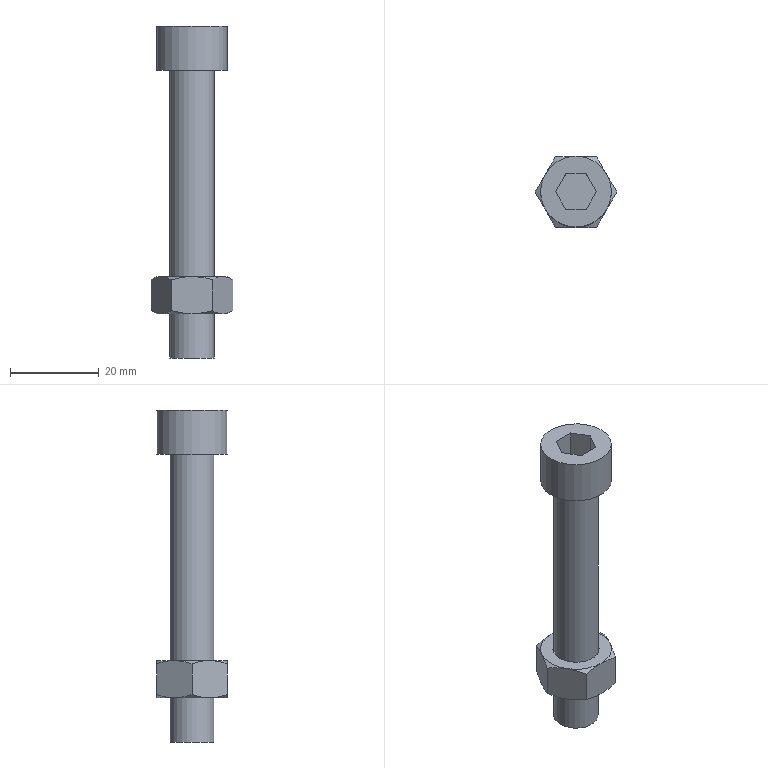Part | STEP file | YBQDJ-YL-13 | 2 solids | 35 faces | box 18.475 x 16 x 75 mm | volume 8074 mm3 | plane 18 | cone 14 | cylinder 3 | commonest cylinder face diameters 8.782 x1 10 x1 16 x1